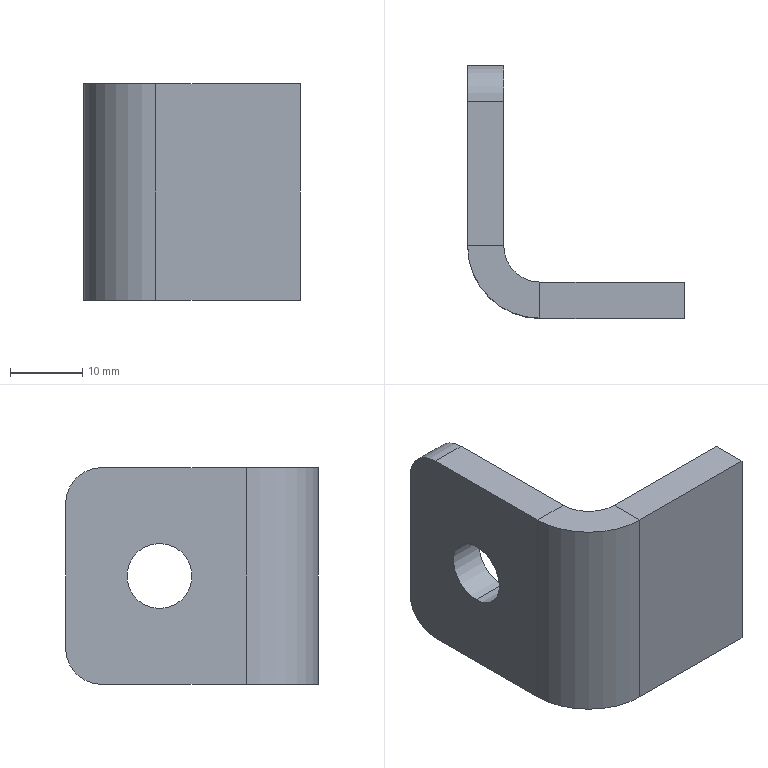Part | SolidWorks | features BaseBody 1, FlatPattern 1, SheetMetal 1, SolidToSheetMetal 1 | 1 solid | 18 faces | box 30 x 35 x 30 mm | volume 8145 mm3 | plane 12 | cylinder 6 | commonest cylinder face diameters 10 x3 9 x2 20 x1
STEP:
#1=CARTESIAN_POINT('',(0.,22.,4.5));
#2=VERTEX_POINT('',#1);
#3=CARTESIAN_POINT('',(5.,22.,4.5));
#4=VERTEX_POINT('',#3);
#5=CARTESIAN_POINT('',(5.,22.,4.5));
#6=DIRECTION('',(1.,0.,0.));
#7=VECTOR('',#6,1000.);
#8=LINE('',#5,#7);
#9=EDGE_CURVE('',#2,#4,#8,.T.);
#10=ORIENTED_EDGE('',*,*,#9,.F.);
#11=CARTESIAN_POINT('',(0.,22.,-4.5));
#12=VERTEX_POINT('',#11);
#13=CARTESIAN_POINT('',(0.,22.,0.));
#14=DIRECTION('',(1.,0.,0.));
#15=DIRECTION('',(0.,0.,-1.));
#16=AXIS2_PLACEMENT_3D('',#13,#14,#15);
#17=CIRCLE('',#16,4.5);
#18=EDGE_CURVE('',#12,#2,#17,.T.);
#19=ORIENTED_EDGE('',*,*,#18,.F.);
#20=CARTESIAN_POINT('',(5.,22.,-4.5));
#21=VERTEX_POINT('',#20);
#22=CARTESIAN_POINT('',(5.,22.,-4.5));
#23=DIRECTION('',(1.,0.,0.));
#24=VECTOR('',#23,1000.);
#25=LINE('',#22,#24);
#26=EDGE_CURVE('',#12,#21,#25,.T.);
#27=ORIENTED_EDGE('',*,*,#26,.T.);
#28=CARTESIAN_POINT('',(5.,22.,0.));
#29=DIRECTION('',(1.,0.,0.));
#30=DIRECTION('',(0.,0.,-1.));
#31=AXIS2_PLACEMENT_3D('',#28,#29,#30);
#32=CIRCLE('',#31,4.5);
#33=EDGE_CURVE('',#21,#4,#32,.T.);
#34=ORIENTED_EDGE('',*,*,#33,.T.);
#35=EDGE_LOOP('',(#10,#19,#27,#34));
#36=FACE_OUTER_BOUND('',#35,.T.);
#37=CARTESIAN_POINT('',(5.,22.,0.));
#38=DIRECTION('',(-1.,0.,0.));
#39=DIRECTION('',(0.,0.,1.));
#40=AXIS2_PLACEMENT_3D('',#37,#38,#39);
#41=CYLINDRICAL_SURFACE('',#40,4.5);
#42=ADVANCED_FACE('',(#36),#41,.F.);
#43=CARTESIAN_POINT('',(0.,30.,-15.));
#44=VERTEX_POINT('',#43);
#45=CARTESIAN_POINT('',(5.,30.,-15.));
#46=VERTEX_POINT('',#45);
#47=CARTESIAN_POINT('',(5.,30.,-15.));
#48=DIRECTION('',(1.,0.,0.));
#49=VECTOR('',#48,1000.);
#50=LINE('',#47,#49);
#51=EDGE_CURVE('',#44,#46,#50,.T.);
#52=ORIENTED_EDGE('',*,*,#51,.F.);
#53=CARTESIAN_POINT('',(0.,35.,-10.));
#54=VERTEX_POINT('',#53);
#55=CARTESIAN_POINT('',(0.,30.,-10.));
#56=DIRECTION('',(1.,0.,0.));
#57=DIRECTION('',(0.,0.,-1.));
#58=AXIS2_PLACEMENT_3D('',#55,#56,#57);
#59=CIRCLE('',#58,5.);
#60=EDGE_CURVE('',#44,#54,#59,.T.);
#61=ORIENTED_EDGE('',*,*,#60,.T.);
#62=CARTESIAN_POINT('',(5.,35.,-10.));
#63=VERTEX_POINT('',#62);
#64=CARTESIAN_POINT('',(5.,35.,-10.));
#65=DIRECTION('',(1.,0.,0.));
#66=VECTOR('',#65,1000.);
#67=LINE('',#64,#66);
#68=EDGE_CURVE('',#54,#63,#67,.T.);
#69=ORIENTED_EDGE('',*,*,#68,.T.);
#70=CARTESIAN_POINT('',(5.,30.,-10.));
#71=DIRECTION('',(1.,0.,0.));
#72=DIRECTION('',(0.,0.,-1.));
#73=AXIS2_PLACEMENT_3D('',#70,#71,#72);
#74=CIRCLE('',#73,5.);
#75=EDGE_CURVE('',#46,#63,#74,.T.);
#76=ORIENTED_EDGE('',*,*,#75,.F.);
#77=EDGE_LOOP('',(#52,#61,#69,#76));
#78=FACE_OUTER_BOUND('',#77,.T.);
#79=CARTESIAN_POINT('',(5.,30.,-10.));
#80=DIRECTION('',(-1.,0.,0.));
#81=DIRECTION('',(0.,0.,1.));
#82=AXIS2_PLACEMENT_3D('',#79,#80,#81);
#83=CYLINDRICAL_SURFACE('',#82,5.);
#84=ADVANCED_FACE('',(#78),#83,.T.);
#85=ORIENTED_EDGE('',*,*,#68,.F.);
#86=CARTESIAN_POINT('',(0.,35.,10.));
#87=VERTEX_POINT('',#86);
#88=CARTESIAN_POINT('',(0.,35.,-15.));
#89=DIRECTION('',(0.,0.,1.));
#90=VECTOR('',#89,1000.);
#91=LINE('',#88,#90);
#92=EDGE_CURVE('',#54,#87,#91,.T.);
#93=ORIENTED_EDGE('',*,*,#92,.T.);
#94=CARTESIAN_POINT('',(5.,35.,10.));
#95=VERTEX_POINT('',#94);
#96=CARTESIAN_POINT('',(5.,35.,10.));
#97=DIRECTION('',(1.,0.,0.));
#98=VECTOR('',#97,1000.);
#99=LINE('',#96,#98);
#100=EDGE_CURVE('',#87,#95,#99,.T.);
#101=ORIENTED_EDGE('',*,*,#100,.T.);
#102=CARTESIAN_POINT('',(5.,35.,-10.));
#103=DIRECTION('',(0.,0.,1.));
#104=VECTOR('',#103,1000.);
#105=LINE('',#102,#104);
#106=EDGE_CURVE('',#63,#95,#105,.T.);
#107=ORIENTED_EDGE('',*,*,#106,.F.);
#108=EDGE_LOOP('',(#85,#93,#101,#107));
#109=FACE_OUTER_BOUND('',#108,.T.);
#110=CARTESIAN_POINT('',(5.,35.,-10.));
#111=DIRECTION('',(0.,-1.,0.));
#112=DIRECTION('',(0.,0.,1.));
#113=AXIS2_PLACEMENT_3D('',#110,#111,#112);
#114=PLANE('',#113);
#115=ADVANCED_FACE('',(#109),#114,.F.);
#116=ORIENTED_EDGE('',*,*,#100,.F.);
#117=CARTESIAN_POINT('',(0.,30.,15.));
#118=VERTEX_POINT('',#117);
#119=CARTESIAN_POINT('',(0.,30.,10.));
#120=DIRECTION('',(1.,0.,0.));
#121=DIRECTION('',(0.,0.,-1.));
#122=AXIS2_PLACEMENT_3D('',#119,#120,#121);
#123=CIRCLE('',#122,5.);
#124=EDGE_CURVE('',#87,#118,#123,.T.);
#125=ORIENTED_EDGE('',*,*,#124,.T.);
#126=CARTESIAN_POINT('',(5.,30.,15.));
#127=VERTEX_POINT('',#126);
#128=CARTESIAN_POINT('',(5.,30.,15.));
#129=DIRECTION('',(1.,0.,0.));
#130=VECTOR('',#129,1000.);
#131=LINE('',#128,#130);
#132=EDGE_CURVE('',#118,#127,#131,.T.);
#133=ORIENTED_EDGE('',*,*,#132,.T.);
#134=CARTESIAN_POINT('',(5.,30.,10.));
#135=DIRECTION('',(1.,0.,0.));
#136=DIRECTION('',(0.,1.,0.));
#137=AXIS2_PLACEMENT_3D('',#134,#135,#136);
#138=CIRCLE('',#137,5.);
#139=EDGE_CURVE('',#95,#127,#138,.T.);
#140=ORIENTED_EDGE('',*,*,#139,.F.);
#141=EDGE_LOOP('',(#116,#125,#133,#140));
#142=FACE_OUTER_BOUND('',#141,.T.);
#143=CARTESIAN_POINT('',(5.,30.,10.));
#144=DIRECTION('',(-1.,0.,0.));
#145=DIRECTION('',(0.,0.,1.));
#146=AXIS2_PLACEMENT_3D('',#143,#144,#145);
#147=CYLINDRICAL_SURFACE('',#146,5.);
#148=ADVANCED_FACE('',(#142),#147,.T.);
#149=ORIENTED_EDGE('',*,*,#132,.F.);
#150=CARTESIAN_POINT('',(0.,10.,15.));
#151=VERTEX_POINT('',#150);
#152=CARTESIAN_POINT('',(0.,35.,15.));
#153=DIRECTION('',(0.,-1.,0.));
#154=VECTOR('',#153,1000.);
#155=LINE('',#152,#154);
#156=EDGE_CURVE('',#118,#151,#155,.T.);
#157=ORIENTED_EDGE('',*,*,#156,.T.);
#158=CARTESIAN_POINT('',(5.,10.,15.));
#159=VERTEX_POINT('',#158);
#160=CARTESIAN_POINT('',(5.,10.,15.));
#161=DIRECTION('',(1.,0.,0.));
#162=VECTOR('',#161,1000.);
#163=LINE('',#160,#162);
#164=EDGE_CURVE('',#151,#159,#163,.T.);
#165=ORIENTED_EDGE('',*,*,#164,.T.);
#166=CARTESIAN_POINT('',(5.,30.,15.));
#167=DIRECTION('',(0.,-1.,0.));
#168=VECTOR('',#167,1000.);
#169=LINE('',#166,#168);
#170=EDGE_CURVE('',#127,#159,#169,.T.);
#171=ORIENTED_EDGE('',*,*,#170,.F.);
#172=EDGE_LOOP('',(#149,#157,#165,#171));
#173=FACE_OUTER_BOUND('',#172,.T.);
#174=CARTESIAN_POINT('',(5.,30.,15.));
#175=DIRECTION('',(0.,0.,-1.));
#176=DIRECTION('',(0.,-1.,0.));
#177=AXIS2_PLACEMENT_3D('',#174,#175,#176);
#178=PLANE('',#177);
#179=ADVANCED_FACE('',(#173),#178,.F.);
#180=ORIENTED_EDGE('',*,*,#164,.F.);
#181=CARTESIAN_POINT('',(10.,0.,15.));
#182=VERTEX_POINT('',#181);
#183=CARTESIAN_POINT('',(10.,10.,15.));
#184=DIRECTION('',(0.,0.,-1.));
#185=DIRECTION('',(-1.,0.,0.));
#186=AXIS2_PLACEMENT_3D('',#183,#184,#185);
#187=CIRCLE('',#186,10.);
#188=EDGE_CURVE('',#182,#151,#187,.T.);
#189=ORIENTED_EDGE('',*,*,#188,.F.);
#190=CARTESIAN_POINT('',(10.,5.,15.));
#191=VERTEX_POINT('',#190);
#192=CARTESIAN_POINT('',(10.,5.,15.));
#193=DIRECTION('',(0.,1.,0.));
#194=VECTOR('',#193,1000.);
#195=LINE('',#192,#194);
#196=EDGE_CURVE('',#182,#191,#195,.T.);
#197=ORIENTED_EDGE('',*,*,#196,.T.);
#198=CARTESIAN_POINT('',(10.,10.,15.));
#199=DIRECTION('',(0.,0.,-1.));
#200=DIRECTION('',(0.,-1.,0.));
#201=AXIS2_PLACEMENT_3D('',#198,#199,#200);
#202=CIRCLE('',#201,5.);
#203=EDGE_CURVE('',#191,#159,#202,.T.);
#204=ORIENTED_EDGE('',*,*,#203,.T.);
#205=EDGE_LOOP('',(#180,#189,#197,#204));
#206=FACE_OUTER_BOUND('',#205,.T.);
#207=CARTESIAN_POINT('',(10.,10.,15.));
#208=DIRECTION('',(0.,0.,1.));
#209=DIRECTION('',(1.,0.,0.));
#210=AXIS2_PLACEMENT_3D('',#207,#208,#209);
#211=PLANE('',#210);
#212=ADVANCED_FACE('',(#206),#211,.T.);
#213=ORIENTED_EDGE('',*,*,#196,.F.);
#214=CARTESIAN_POINT('',(30.,0.,15.));
#215=VERTEX_POINT('',#214);
#216=CARTESIAN_POINT('',(0.,0.,15.));
#217=DIRECTION('',(1.,0.,0.));
#218=VECTOR('',#217,1000.);
#219=LINE('',#216,#218);
#220=EDGE_CURVE('',#182,#215,#219,.T.);
#221=ORIENTED_EDGE('',*,*,#220,.T.);
#222=CARTESIAN_POINT('',(30.,5.,15.));
#223=VERTEX_POINT('',#222);
#224=CARTESIAN_POINT('',(30.,5.,15.));
#225=DIRECTION('',(0.,1.,0.));
#226=VECTOR('',#225,1000.);
#227=LINE('',#224,#226);
#228=EDGE_CURVE('',#215,#223,#227,.T.);
#229=ORIENTED_EDGE('',*,*,#228,.T.);
#230=CARTESIAN_POINT('',(10.,5.,15.));
#231=DIRECTION('',(1.,0.,0.));
#232=VECTOR('',#231,1000.);
#233=LINE('',#230,#232);
#234=EDGE_CURVE('',#191,#223,#233,.T.);
#235=ORIENTED_EDGE('',*,*,#234,.F.);
#236=EDGE_LOOP('',(#213,#221,#229,#235));
#237=FACE_OUTER_BOUND('',#236,.T.);
#238=CARTESIAN_POINT('',(10.,5.,15.));
#239=DIRECTION('',(0.,0.,-1.));
#240=DIRECTION('',(1.,0.,0.));
#241=AXIS2_PLACEMENT_3D('',#238,#239,#240);
#242=PLANE('',#241);
#243=ADVANCED_FACE('',(#237),#242,.F.);
#244=ORIENTED_EDGE('',*,*,#228,.F.);
#245=CARTESIAN_POINT('',(30.,0.,-15.));
#246=VERTEX_POINT('',#245);
#247=CARTESIAN_POINT('',(30.,0.,-15.));
#248=DIRECTION('',(0.,0.,1.));
#249=VECTOR('',#248,1000.);
#250=LINE('',#247,#249);
#251=EDGE_CURVE('',#246,#215,#250,.T.);
#252=ORIENTED_EDGE('',*,*,#251,.F.);
#253=CARTESIAN_POINT('',(30.,5.,-15.));
#254=VERTEX_POINT('',#253);
#255=CARTESIAN_POINT('',(30.,5.,-15.));
#256=DIRECTION('',(0.,1.,0.));
#257=VECTOR('',#256,1000.);
#258=LINE('',#255,#257);
#259=EDGE_CURVE('',#246,#254,#258,.T.);
#260=ORIENTED_EDGE('',*,*,#259,.T.);
#261=CARTESIAN_POINT('',(30.,5.,-15.));
#262=DIRECTION('',(0.,0.,1.));
#263=VECTOR('',#262,1000.);
#264=LINE('',#261,#263);
#265=EDGE_CURVE('',#254,#223,#264,.T.);
#266=ORIENTED_EDGE('',*,*,#265,.T.);
#267=EDGE_LOOP('',(#244,#252,#260,#266));
#268=FACE_OUTER_BOUND('',#267,.T.);
#269=CARTESIAN_POINT('',(30.,5.,-15.));
#270=DIRECTION('',(1.,0.,0.));
#271=DIRECTION('',(0.,0.,1.));
#272=AXIS2_PLACEMENT_3D('',#269,#270,#271);
#273=PLANE('',#272);
#274=ADVANCED_FACE('',(#268),#273,.T.);
#275=ORIENTED_EDGE('',*,*,#259,.F.);
#276=CARTESIAN_POINT('',(10.,0.,-15.));
#277=VERTEX_POINT('',#276);
#278=CARTESIAN_POINT('',(0.,0.,-15.));
#279=DIRECTION('',(1.,0.,0.));
#280=VECTOR('',#279,1000.);
#281=LINE('',#278,#280);
#282=EDGE_CURVE('',#277,#246,#281,.T.);
#283=ORIENTED_EDGE('',*,*,#282,.F.);
#284=CARTESIAN_POINT('',(10.,5.,-15.));
#285=VERTEX_POINT('',#284);
#286=CARTESIAN_POINT('',(10.,5.,-15.));
#287=DIRECTION('',(0.,1.,0.));
#288=VECTOR('',#287,1000.);
#289=LINE('',#286,#288);
#290=EDGE_CURVE('',#277,#285,#289,.T.);
#291=ORIENTED_EDGE('',*,*,#290,.T.);
#292=CARTESIAN_POINT('',(10.,5.,-15.));
#293=DIRECTION('',(1.,0.,0.));
#294=VECTOR('',#293,1000.);
#295=LINE('',#292,#294);
#296=EDGE_CURVE('',#285,#254,#295,.T.);
#297=ORIENTED_EDGE('',*,*,#296,.T.);
#298=EDGE_LOOP('',(#275,#283,#291,#297));
#299=FACE_OUTER_BOUND('',#298,.T.);
#300=CARTESIAN_POINT('',(10.,5.,-15.));
#301=DIRECTION('',(0.,0.,-1.));
#302=DIRECTION('',(1.,0.,0.));
#303=AXIS2_PLACEMENT_3D('',#300,#301,#302);
#304=PLANE('',#303);
#305=ADVANCED_FACE('',(#299),#304,.T.);
#306=ORIENTED_EDGE('',*,*,#290,.F.);
#307=CARTESIAN_POINT('',(0.,10.,-15.));
#308=VERTEX_POINT('',#307);
#309=CARTESIAN_POINT('',(10.,10.,-15.));
#310=DIRECTION('',(0.,0.,-1.));
#311=DIRECTION('',(-1.,0.,0.));
#312=AXIS2_PLACEMENT_3D('',#309,#310,#311);
#313=CIRCLE('',#312,10.);
#314=EDGE_CURVE('',#277,#308,#313,.T.);
#315=ORIENTED_EDGE('',*,*,#314,.T.);
#316=CARTESIAN_POINT('',(5.,10.,-15.));
#317=VERTEX_POINT('',#316);
#318=CARTESIAN_POINT('',(5.,10.,-15.));
#319=DIRECTION('',(1.,0.,0.));
#320=VECTOR('',#319,1000.);
#321=LINE('',#318,#320);
#322=EDGE_CURVE('',#308,#317,#321,.T.);
#323=ORIENTED_EDGE('',*,*,#322,.T.);
#324=CARTESIAN_POINT('',(10.,10.,-15.));
#325=DIRECTION('',(0.,0.,-1.));
#326=DIRECTION('',(0.,-1.,0.));
#327=AXIS2_PLACEMENT_3D('',#324,#325,#326);
#328=CIRCLE('',#327,5.);
#329=EDGE_CURVE('',#285,#317,#328,.T.);
#330=ORIENTED_EDGE('',*,*,#329,.F.);
#331=EDGE_LOOP('',(#306,#315,#323,#330));
#332=FACE_OUTER_BOUND('',#331,.T.);
#333=CARTESIAN_POINT('',(10.,10.,-15.));
#334=DIRECTION('',(0.,0.,1.));
#335=DIRECTION('',(1.,0.,0.));
#336=AXIS2_PLACEMENT_3D('',#333,#334,#335);
#337=PLANE('',#336);
#338=ADVANCED_FACE('',(#332),#337,.F.);
#339=CARTESIAN_POINT('',(0.,22.,0.));
#340=DIRECTION('',(1.,0.,0.));
#341=DIRECTION('',(0.,0.,-1.));
#342=AXIS2_PLACEMENT_3D('',#339,#340,#341);
#343=CIRCLE('',#342,4.5);
#344=EDGE_CURVE('',#2,#12,#343,.T.);
#345=ORIENTED_EDGE('',*,*,#344,.F.);
#346=ORIENTED_EDGE('',*,*,#9,.T.);
#347=CARTESIAN_POINT('',(5.,22.,0.));
#348=DIRECTION('',(1.,0.,0.));
#349=DIRECTION('',(0.,0.,1.));
#350=AXIS2_PLACEMENT_3D('',#347,#348,#349);
#351=CIRCLE('',#350,4.5);
#352=EDGE_CURVE('',#4,#21,#351,.T.);
#353=ORIENTED_EDGE('',*,*,#352,.T.);
#354=ORIENTED_EDGE('',*,*,#26,.F.);
#355=EDGE_LOOP('',(#345,#346,#353,#354));
#356=FACE_OUTER_BOUND('',#355,.T.);
#357=CARTESIAN_POINT('',(5.,22.,0.));
#358=DIRECTION('',(-1.,0.,0.));
#359=DIRECTION('',(0.,0.,1.));
#360=AXIS2_PLACEMENT_3D('',#357,#358,#359);
#361=CYLINDRICAL_SURFACE('',#360,4.5);
#362=ADVANCED_FACE('',(#356),#361,.F.);
#363=CARTESIAN_POINT('',(0.,35.,-15.));
#364=DIRECTION('',(0.,-1.,0.));
#365=VECTOR('',#364,1000.);
#366=LINE('',#363,#365);
#367=EDGE_CURVE('',#44,#308,#366,.T.);
#368=ORIENTED_EDGE('',*,*,#367,.F.);
#369=ORIENTED_EDGE('',*,*,#51,.T.);
#370=CARTESIAN_POINT('',(5.,30.,-15.));
#371=DIRECTION('',(0.,-1.,0.));
#372=VECTOR('',#371,1000.);
#373=LINE('',#370,#372);
#374=EDGE_CURVE('',#46,#317,#373,.T.);
#375=ORIENTED_EDGE('',*,*,#374,.T.);
#376=ORIENTED_EDGE('',*,*,#322,.F.);
#377=EDGE_LOOP('',(#368,#369,#375,#376));
#378=FACE_OUTER_BOUND('',#377,.T.);
#379=CARTESIAN_POINT('',(5.,30.,-15.));
#380=DIRECTION('',(0.,0.,-1.));
#381=DIRECTION('',(0.,-1.,0.));
#382=AXIS2_PLACEMENT_3D('',#379,#380,#381);
#383=PLANE('',#382);
#384=ADVANCED_FACE('',(#378),#383,.T.);
#385=ORIENTED_EDGE('',*,*,#329,.T.);
#386=CARTESIAN_POINT('',(5.,10.,-15.));
#387=DIRECTION('',(0.,0.,1.));
#388=VECTOR('',#387,1000.);
#389=LINE('',#386,#388);
#390=EDGE_CURVE('',#317,#159,#389,.T.);
#391=ORIENTED_EDGE('',*,*,#390,.T.);
#392=ORIENTED_EDGE('',*,*,#203,.F.);
#393=CARTESIAN_POINT('',(10.,5.,-15.));
#394=DIRECTION('',(0.,0.,1.));
#395=VECTOR('',#394,1000.);
#396=LINE('',#393,#395);
#397=EDGE_CURVE('',#285,#191,#396,.T.);
#398=ORIENTED_EDGE('',*,*,#397,.F.);
#399=EDGE_LOOP('',(#385,#391,#392,#398));
#400=FACE_OUTER_BOUND('',#399,.T.);
#401=CARTESIAN_POINT('',(10.,10.,-15.));
#402=DIRECTION('',(0.,0.,-1.));
#403=DIRECTION('',(0.,-1.,0.));
#404=AXIS2_PLACEMENT_3D('',#401,#402,#403);
#405=CYLINDRICAL_SURFACE('',#404,5.);
#406=ADVANCED_FACE('',(#400),#405,.F.);
#407=ORIENTED_EDGE('',*,*,#397,.T.);
#408=ORIENTED_EDGE('',*,*,#234,.T.);
#409=ORIENTED_EDGE('',*,*,#265,.F.);
#410=ORIENTED_EDGE('',*,*,#296,.F.);
#411=EDGE_LOOP('',(#407,#408,#409,#410));
#412=FACE_OUTER_BOUND('',#411,.T.);
#413=CARTESIAN_POINT('',(0.,5.,-15.));
#414=DIRECTION('',(0.,-1.,0.));
#415=DIRECTION('',(0.,0.,-1.));
#416=AXIS2_PLACEMENT_3D('',#413,#414,#415);
#417=PLANE('',#416);
#418=ADVANCED_FACE('',(#412),#417,.F.);
#419=ORIENTED_EDGE('',*,*,#170,.T.);
#420=ORIENTED_EDGE('',*,*,#390,.F.);
#421=ORIENTED_EDGE('',*,*,#374,.F.);
#422=ORIENTED_EDGE('',*,*,#75,.T.);
#423=ORIENTED_EDGE('',*,*,#106,.T.);
#424=ORIENTED_EDGE('',*,*,#139,.T.);
#425=EDGE_LOOP('',(#419,#420,#421,#422,#423,#424));
#426=FACE_OUTER_BOUND('',#425,.T.);
#427=ORIENTED_EDGE('',*,*,#33,.F.);
#428=ORIENTED_EDGE('',*,*,#352,.F.);
#429=EDGE_LOOP('',(#427,#428));
#430=FACE_BOUND('',#429,.T.);
#431=CARTESIAN_POINT('',(5.,35.,-15.));
#432=DIRECTION('',(-1.,0.,0.));
#433=DIRECTION('',(0.,0.,1.));
#434=AXIS2_PLACEMENT_3D('',#431,#432,#433);
#435=PLANE('',#434);
#436=ADVANCED_FACE('',(#426,#430),#435,.F.);
#437=ORIENTED_EDGE('',*,*,#314,.F.);
#438=CARTESIAN_POINT('',(10.,0.,-15.));
#439=DIRECTION('',(0.,0.,1.));
#440=VECTOR('',#439,1000.);
#441=LINE('',#438,#440);
#442=EDGE_CURVE('',#277,#182,#441,.T.);
#443=ORIENTED_EDGE('',*,*,#442,.T.);
#444=ORIENTED_EDGE('',*,*,#188,.T.);
#445=CARTESIAN_POINT('',(0.,10.,-15.));
#446=DIRECTION('',(0.,0.,1.));
#447=VECTOR('',#446,1000.);
#448=LINE('',#445,#447);
#449=EDGE_CURVE('',#308,#151,#448,.T.);
#450=ORIENTED_EDGE('',*,*,#449,.F.);
#451=EDGE_LOOP('',(#437,#443,#444,#450));
#452=FACE_OUTER_BOUND('',#451,.T.);
#453=CARTESIAN_POINT('',(10.,10.,-15.));
#454=DIRECTION('',(0.,0.,-1.));
#455=DIRECTION('',(0.,-1.,0.));
#456=AXIS2_PLACEMENT_3D('',#453,#454,#455);
#457=CYLINDRICAL_SURFACE('',#456,10.);
#458=ADVANCED_FACE('',(#452),#457,.T.);
#459=ORIENTED_EDGE('',*,*,#442,.F.);
#460=ORIENTED_EDGE('',*,*,#282,.T.);
#461=ORIENTED_EDGE('',*,*,#251,.T.);
#462=ORIENTED_EDGE('',*,*,#220,.F.);
#463=EDGE_LOOP('',(#459,#460,#461,#462));
#464=FACE_OUTER_BOUND('',#463,.T.);
#465=CARTESIAN_POINT('',(0.,0.,-15.));
#466=DIRECTION('',(0.,-1.,0.));
#467=DIRECTION('',(0.,0.,-1.));
#468=AXIS2_PLACEMENT_3D('',#465,#466,#467);
#469=PLANE('',#468);
#470=ADVANCED_FACE('',(#464),#469,.T.);
#471=ORIENTED_EDGE('',*,*,#156,.F.);
#472=ORIENTED_EDGE('',*,*,#124,.F.);
#473=ORIENTED_EDGE('',*,*,#92,.F.);
#474=ORIENTED_EDGE('',*,*,#60,.F.);
#475=ORIENTED_EDGE('',*,*,#367,.T.);
#476=ORIENTED_EDGE('',*,*,#449,.T.);
#477=EDGE_LOOP('',(#471,#472,#473,#474,#475,#476));
#478=FACE_OUTER_BOUND('',#477,.T.);
#479=ORIENTED_EDGE('',*,*,#18,.T.);
#480=ORIENTED_EDGE('',*,*,#344,.T.);
#481=EDGE_LOOP('',(#479,#480));
#482=FACE_BOUND('',#481,.T.);
#483=CARTESIAN_POINT('',(0.,35.,-15.));
#484=DIRECTION('',(-1.,0.,0.));
#485=DIRECTION('',(0.,0.,1.));
#486=AXIS2_PLACEMENT_3D('',#483,#484,#485);
#487=PLANE('',#486);
#488=ADVANCED_FACE('',(#478,#482),#487,.T.);
#489=CLOSED_SHELL('',(#42,#84,#115,#148,#179,#212,#243,#274,#305,#338,#362,#384,#406,#418,#436,#458,#470,#488));
#490=MANIFOLD_SOLID_BREP('',#489);
#491=CARTESIAN_POINT('',(0.,0.,0.));
#492=DIRECTION('',(0.,0.,1.));
#493=DIRECTION('',(1.,0.,0.));
#494=AXIS2_PLACEMENT_3D('',#491,#492,#493);
#495=(LENGTH_UNIT()NAMED_UNIT(*)SI_UNIT(.MILLI.,.METRE.));
#496=UNCERTAINTY_MEASURE_WITH_UNIT(LENGTH_MEASURE(0.00001),#495,'','');
#497=(NAMED_UNIT(*)PLANE_ANGLE_UNIT()SI_UNIT($,.RADIAN.));
#498=(NAMED_UNIT(*)SI_UNIT($,.STERADIAN.)SOLID_ANGLE_UNIT());
#499=(GEOMETRIC_REPRESENTATION_CONTEXT(3)GLOBAL_UNCERTAINTY_ASSIGNED_CONTEXT((#496))GLOBAL_UNIT_ASSIGNED_CONTEXT((#495,#497,#498))REPRESENTATION_CONTEXT('',''));
#500=ADVANCED_BREP_SHAPE_REPRESENTATION('',(#490,#494),#499);